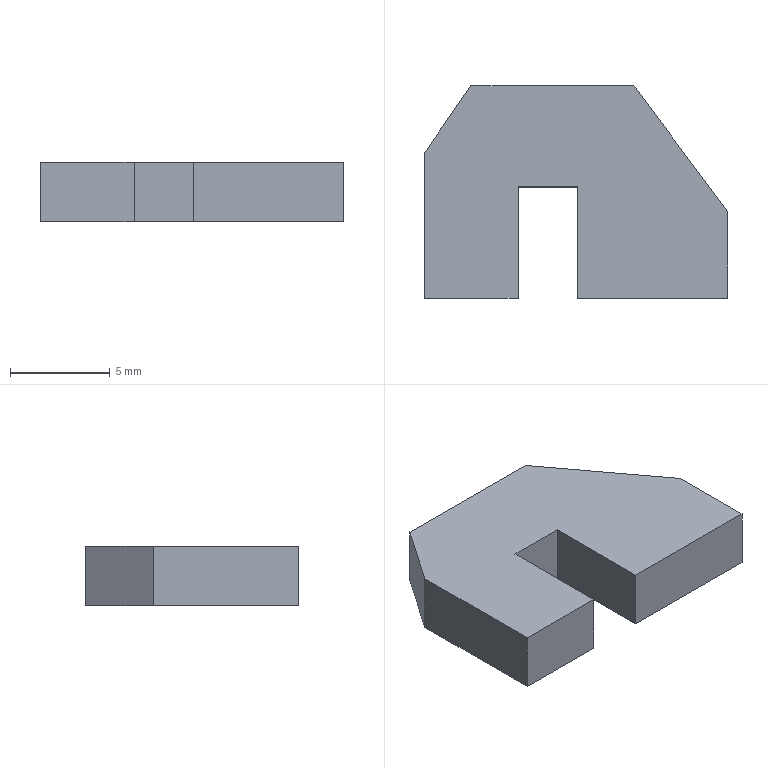Part | SolidWorks | features BaseBody 1 | 1 solid | 12 faces | box 15.248 x 10.684 x 3 mm | volume 381.769 mm3 | plane 10 | spline 2
STEP:
#1=CARTESIAN_POINT('',(96.385,5.305,-1.5));
#2=VERTEX_POINT('',#1);
#3=CARTESIAN_POINT('',(96.385,10.901,-1.5));
#4=VERTEX_POINT('',#3);
#5=CARTESIAN_POINT('',(96.385,0.,-1.5));
#6=DIRECTION('',(0.,1.,0.));
#7=VECTOR('',#6,1000.);
#8=LINE('',#5,#7);
#9=EDGE_CURVE('',#2,#4,#8,.T.);
#10=ORIENTED_EDGE('',*,*,#9,.T.);
#11=CARTESIAN_POINT('',(93.391,10.901,-1.5));
#12=VERTEX_POINT('',#11);
#13=CARTESIAN_POINT('',(0.,10.901,-1.5));
#14=DIRECTION('',(-1.,0.,0.));
#15=VECTOR('',#14,1000.);
#16=LINE('',#13,#15);
#17=EDGE_CURVE('',#4,#12,#16,.T.);
#18=ORIENTED_EDGE('',*,*,#17,.T.);
#19=CARTESIAN_POINT('',(93.391,5.305,-1.5));
#20=VERTEX_POINT('',#19);
#21=CARTESIAN_POINT('',(93.391,0.,-1.5));
#22=DIRECTION('',(0.,-1.,0.));
#23=VECTOR('',#22,1000.);
#24=LINE('',#21,#23);
#25=EDGE_CURVE('',#12,#20,#24,.T.);
#26=ORIENTED_EDGE('',*,*,#25,.T.);
#27=CARTESIAN_POINT('',(88.677,5.305,-1.5));
#28=VERTEX_POINT('',#27);
#29=CARTESIAN_POINT('',(0.,5.305,-1.5));
#30=DIRECTION('',(1.,0.,0.));
#31=VECTOR('',#30,1000.);
#32=LINE('',#29,#31);
#33=EDGE_CURVE('',#28,#20,#32,.T.);
#34=ORIENTED_EDGE('',*,*,#33,.F.);
#35=CARTESIAN_POINT('',(88.677,12.595,-1.5));
#36=VERTEX_POINT('',#35);
#37=CARTESIAN_POINT('',(88.677,0.,-1.5));
#38=DIRECTION('',(0.,-1.,0.));
#39=VECTOR('',#38,1000.);
#40=LINE('',#37,#39);
#41=EDGE_CURVE('',#36,#28,#40,.T.);
#42=ORIENTED_EDGE('',*,*,#41,.F.);
#43=CARTESIAN_POINT('',(91.019,15.989,-1.5));
#44=VERTEX_POINT('',#43);
#45=CARTESIAN_POINT('',(91.019,15.989,-1.5));
#46=CARTESIAN_POINT('',(90.238,14.856,-1.5));
#47=CARTESIAN_POINT('',(89.458,13.725,-1.5));
#48=CARTESIAN_POINT('',(88.677,12.595,-1.5));
#49=B_SPLINE_CURVE_WITH_KNOTS('',3,(#45,#46,#47,#48),.UNSPECIFIED.,.F.,.F.,(4,4),(0.7273,0.8182),.UNSPECIFIED.);
#50=EDGE_CURVE('',#44,#36,#49,.T.);
#51=ORIENTED_EDGE('',*,*,#50,.F.);
#52=CARTESIAN_POINT('',(99.205,15.989,-1.5));
#53=VERTEX_POINT('',#52);
#54=CARTESIAN_POINT('',(0.,15.989,-1.5));
#55=DIRECTION('',(-1.,0.,0.));
#56=VECTOR('',#55,1000.);
#57=LINE('',#54,#56);
#58=EDGE_CURVE('',#53,#44,#57,.T.);
#59=ORIENTED_EDGE('',*,*,#58,.F.);
#60=CARTESIAN_POINT('',(103.925,9.662,-1.5));
#61=VERTEX_POINT('',#60);
#62=CARTESIAN_POINT('',(103.925,9.662,-1.5));
#63=CARTESIAN_POINT('',(102.352,11.771,-1.5));
#64=CARTESIAN_POINT('',(100.779,13.879,-1.5));
#65=CARTESIAN_POINT('',(99.205,15.989,-1.5));
#66=B_SPLINE_CURVE_WITH_KNOTS('',3,(#62,#63,#64,#65),.UNSPECIFIED.,.F.,.F.,(4,4),(0.5455,0.6364),.UNSPECIFIED.);
#67=EDGE_CURVE('',#61,#53,#66,.T.);
#68=ORIENTED_EDGE('',*,*,#67,.F.);
#69=CARTESIAN_POINT('',(103.925,5.305,-1.5));
#70=VERTEX_POINT('',#69);
#71=CARTESIAN_POINT('',(103.925,0.,-1.5));
#72=DIRECTION('',(0.,1.,0.));
#73=VECTOR('',#72,1000.);
#74=LINE('',#71,#73);
#75=EDGE_CURVE('',#70,#61,#74,.T.);
#76=ORIENTED_EDGE('',*,*,#75,.F.);
#77=CARTESIAN_POINT('',(0.,5.305,-1.5));
#78=DIRECTION('',(1.,0.,0.));
#79=VECTOR('',#78,1000.);
#80=LINE('',#77,#79);
#81=EDGE_CURVE('',#2,#70,#80,.T.);
#82=ORIENTED_EDGE('',*,*,#81,.F.);
#83=EDGE_LOOP('',(#10,#18,#26,#34,#42,#51,#59,#68,#76,#82));
#84=FACE_OUTER_BOUND('',#83,.T.);
#85=CARTESIAN_POINT('',(0.,0.,-1.5));
#86=DIRECTION('',(0.,0.,1.));
#87=DIRECTION('',(1.,0.,0.));
#88=AXIS2_PLACEMENT_3D('',#85,#86,#87);
#89=PLANE('',#88);
#90=ADVANCED_FACE('',(#84),#89,.F.);
#91=CARTESIAN_POINT('',(96.385,5.305,1.5));
#92=VERTEX_POINT('',#91);
#93=CARTESIAN_POINT('',(96.385,10.901,1.5));
#94=VERTEX_POINT('',#93);
#95=CARTESIAN_POINT('',(96.385,0.,1.5));
#96=DIRECTION('',(0.,1.,0.));
#97=VECTOR('',#96,1000.);
#98=LINE('',#95,#97);
#99=EDGE_CURVE('',#92,#94,#98,.T.);
#100=ORIENTED_EDGE('',*,*,#99,.F.);
#101=CARTESIAN_POINT('',(103.925,5.305,1.5));
#102=VERTEX_POINT('',#101);
#103=CARTESIAN_POINT('',(0.,5.305,1.5));
#104=DIRECTION('',(1.,0.,0.));
#105=VECTOR('',#104,1000.);
#106=LINE('',#103,#105);
#107=EDGE_CURVE('',#92,#102,#106,.T.);
#108=ORIENTED_EDGE('',*,*,#107,.T.);
#109=CARTESIAN_POINT('',(103.925,9.662,1.5));
#110=VERTEX_POINT('',#109);
#111=CARTESIAN_POINT('',(103.925,0.,1.5));
#112=DIRECTION('',(0.,1.,0.));
#113=VECTOR('',#112,1000.);
#114=LINE('',#111,#113);
#115=EDGE_CURVE('',#102,#110,#114,.T.);
#116=ORIENTED_EDGE('',*,*,#115,.T.);
#117=CARTESIAN_POINT('',(99.205,15.989,1.5));
#118=VERTEX_POINT('',#117);
#119=CARTESIAN_POINT('',(103.925,9.662,1.5));
#120=CARTESIAN_POINT('',(102.352,11.771,1.5));
#121=CARTESIAN_POINT('',(100.779,13.879,1.5));
#122=CARTESIAN_POINT('',(99.205,15.989,1.5));
#123=B_SPLINE_CURVE_WITH_KNOTS('',3,(#119,#120,#121,#122),.UNSPECIFIED.,.F.,.F.,(4,4),(0.5455,0.6364),.UNSPECIFIED.);
#124=EDGE_CURVE('',#110,#118,#123,.T.);
#125=ORIENTED_EDGE('',*,*,#124,.T.);
#126=CARTESIAN_POINT('',(91.019,15.989,1.5));
#127=VERTEX_POINT('',#126);
#128=CARTESIAN_POINT('',(0.,15.989,1.5));
#129=DIRECTION('',(-1.,0.,0.));
#130=VECTOR('',#129,1000.);
#131=LINE('',#128,#130);
#132=EDGE_CURVE('',#118,#127,#131,.T.);
#133=ORIENTED_EDGE('',*,*,#132,.T.);
#134=CARTESIAN_POINT('',(88.677,12.595,1.5));
#135=VERTEX_POINT('',#134);
#136=CARTESIAN_POINT('',(91.019,15.989,1.5));
#137=CARTESIAN_POINT('',(90.238,14.856,1.5));
#138=CARTESIAN_POINT('',(89.458,13.725,1.5));
#139=CARTESIAN_POINT('',(88.677,12.595,1.5));
#140=B_SPLINE_CURVE_WITH_KNOTS('',3,(#136,#137,#138,#139),.UNSPECIFIED.,.F.,.F.,(4,4),(0.7273,0.8182),.UNSPECIFIED.);
#141=EDGE_CURVE('',#127,#135,#140,.T.);
#142=ORIENTED_EDGE('',*,*,#141,.T.);
#143=CARTESIAN_POINT('',(88.677,5.305,1.5));
#144=VERTEX_POINT('',#143);
#145=CARTESIAN_POINT('',(88.677,0.,1.5));
#146=DIRECTION('',(0.,-1.,0.));
#147=VECTOR('',#146,1000.);
#148=LINE('',#145,#147);
#149=EDGE_CURVE('',#135,#144,#148,.T.);
#150=ORIENTED_EDGE('',*,*,#149,.T.);
#151=CARTESIAN_POINT('',(93.391,5.305,1.5));
#152=VERTEX_POINT('',#151);
#153=CARTESIAN_POINT('',(0.,5.305,1.5));
#154=DIRECTION('',(1.,0.,0.));
#155=VECTOR('',#154,1000.);
#156=LINE('',#153,#155);
#157=EDGE_CURVE('',#144,#152,#156,.T.);
#158=ORIENTED_EDGE('',*,*,#157,.T.);
#159=CARTESIAN_POINT('',(93.391,10.901,1.5));
#160=VERTEX_POINT('',#159);
#161=CARTESIAN_POINT('',(93.391,0.,1.5));
#162=DIRECTION('',(0.,-1.,0.));
#163=VECTOR('',#162,1000.);
#164=LINE('',#161,#163);
#165=EDGE_CURVE('',#160,#152,#164,.T.);
#166=ORIENTED_EDGE('',*,*,#165,.F.);
#167=CARTESIAN_POINT('',(0.,10.901,1.5));
#168=DIRECTION('',(-1.,0.,0.));
#169=VECTOR('',#168,1000.);
#170=LINE('',#167,#169);
#171=EDGE_CURVE('',#94,#160,#170,.T.);
#172=ORIENTED_EDGE('',*,*,#171,.F.);
#173=EDGE_LOOP('',(#100,#108,#116,#125,#133,#142,#150,#158,#166,#172));
#174=FACE_OUTER_BOUND('',#173,.T.);
#175=CARTESIAN_POINT('',(0.,0.,1.5));
#176=DIRECTION('',(0.,0.,1.));
#177=DIRECTION('',(1.,0.,0.));
#178=AXIS2_PLACEMENT_3D('',#175,#176,#177);
#179=PLANE('',#178);
#180=ADVANCED_FACE('',(#174),#179,.T.);
#181=ORIENTED_EDGE('',*,*,#17,.F.);
#182=CARTESIAN_POINT('',(96.385,10.901,1.5));
#183=DIRECTION('',(0.,0.,-1.));
#184=VECTOR('',#183,1000.);
#185=LINE('',#182,#184);
#186=EDGE_CURVE('',#94,#4,#185,.T.);
#187=ORIENTED_EDGE('',*,*,#186,.F.);
#188=ORIENTED_EDGE('',*,*,#171,.T.);
#189=CARTESIAN_POINT('',(93.391,10.901,1.5));
#190=DIRECTION('',(0.,0.,-1.));
#191=VECTOR('',#190,1000.);
#192=LINE('',#189,#191);
#193=EDGE_CURVE('',#160,#12,#192,.T.);
#194=ORIENTED_EDGE('',*,*,#193,.T.);
#195=EDGE_LOOP('',(#181,#187,#188,#194));
#196=FACE_OUTER_BOUND('',#195,.T.);
#197=CARTESIAN_POINT('',(0.,10.901,1.5));
#198=DIRECTION('',(0.,-1.,0.));
#199=DIRECTION('',(0.,0.,-1.));
#200=AXIS2_PLACEMENT_3D('',#197,#198,#199);
#201=PLANE('',#200);
#202=ADVANCED_FACE('',(#196),#201,.T.);
#203=ORIENTED_EDGE('',*,*,#25,.F.);
#204=ORIENTED_EDGE('',*,*,#193,.F.);
#205=ORIENTED_EDGE('',*,*,#165,.T.);
#206=CARTESIAN_POINT('',(93.391,5.305,1.5));
#207=DIRECTION('',(0.,0.,-1.));
#208=VECTOR('',#207,1000.);
#209=LINE('',#206,#208);
#210=EDGE_CURVE('',#152,#20,#209,.T.);
#211=ORIENTED_EDGE('',*,*,#210,.T.);
#212=EDGE_LOOP('',(#203,#204,#205,#211));
#213=FACE_OUTER_BOUND('',#212,.T.);
#214=CARTESIAN_POINT('',(93.391,0.,1.5));
#215=DIRECTION('',(1.,0.,0.));
#216=DIRECTION('',(0.,1.,0.));
#217=AXIS2_PLACEMENT_3D('',#214,#215,#216);
#218=PLANE('',#217);
#219=ADVANCED_FACE('',(#213),#218,.T.);
#220=ORIENTED_EDGE('',*,*,#33,.T.);
#221=ORIENTED_EDGE('',*,*,#210,.F.);
#222=ORIENTED_EDGE('',*,*,#157,.F.);
#223=CARTESIAN_POINT('',(88.677,5.305,1.5));
#224=DIRECTION('',(0.,0.,-1.));
#225=VECTOR('',#224,1000.);
#226=LINE('',#223,#225);
#227=EDGE_CURVE('',#144,#28,#226,.T.);
#228=ORIENTED_EDGE('',*,*,#227,.T.);
#229=EDGE_LOOP('',(#220,#221,#222,#228));
#230=FACE_OUTER_BOUND('',#229,.T.);
#231=CARTESIAN_POINT('',(0.,5.305,1.5));
#232=DIRECTION('',(0.,1.,0.));
#233=DIRECTION('',(1.,0.,0.));
#234=AXIS2_PLACEMENT_3D('',#231,#232,#233);
#235=PLANE('',#234);
#236=ADVANCED_FACE('',(#230),#235,.F.);
#237=ORIENTED_EDGE('',*,*,#41,.T.);
#238=ORIENTED_EDGE('',*,*,#227,.F.);
#239=ORIENTED_EDGE('',*,*,#149,.F.);
#240=CARTESIAN_POINT('',(88.677,12.595,1.5));
#241=DIRECTION('',(0.,0.,-1.));
#242=VECTOR('',#241,1000.);
#243=LINE('',#240,#242);
#244=EDGE_CURVE('',#135,#36,#243,.T.);
#245=ORIENTED_EDGE('',*,*,#244,.T.);
#246=EDGE_LOOP('',(#237,#238,#239,#245));
#247=FACE_OUTER_BOUND('',#246,.T.);
#248=CARTESIAN_POINT('',(88.677,0.,1.5));
#249=DIRECTION('',(1.,0.,0.));
#250=DIRECTION('',(0.,1.,0.));
#251=AXIS2_PLACEMENT_3D('',#248,#249,#250);
#252=PLANE('',#251);
#253=ADVANCED_FACE('',(#247),#252,.F.);
#254=ORIENTED_EDGE('',*,*,#50,.T.);
#255=ORIENTED_EDGE('',*,*,#244,.F.);
#256=ORIENTED_EDGE('',*,*,#141,.F.);
#257=CARTESIAN_POINT('',(91.019,15.989,1.5));
#258=DIRECTION('',(0.,0.,-1.));
#259=VECTOR('',#258,1000.);
#260=LINE('',#257,#259);
#261=EDGE_CURVE('',#127,#44,#260,.T.);
#262=ORIENTED_EDGE('',*,*,#261,.T.);
#263=EDGE_LOOP('',(#254,#255,#256,#262));
#264=FACE_OUTER_BOUND('',#263,.T.);
#265=CARTESIAN_POINT('',(91.019,15.989,1.5));
#266=CARTESIAN_POINT('',(91.019,15.989,-1.5));
#267=CARTESIAN_POINT('',(90.238,14.856,1.5));
#268=CARTESIAN_POINT('',(90.238,14.856,-1.5));
#269=CARTESIAN_POINT('',(89.458,13.725,1.5));
#270=CARTESIAN_POINT('',(89.458,13.725,-1.5));
#271=CARTESIAN_POINT('',(88.677,12.595,1.5));
#272=CARTESIAN_POINT('',(88.677,12.595,-1.5));
#273=B_SPLINE_SURFACE_WITH_KNOTS('',3,1,((#265,#266),(#267,#268),(#269,#270),(#271,#272)),.UNSPECIFIED.,.F.,.F.,.F.,(4,4),(2,2),(0.7273,0.8182),(0.,1.),.UNSPECIFIED.);
#274=ADVANCED_FACE('',(#264),#273,.F.);
#275=ORIENTED_EDGE('',*,*,#58,.T.);
#276=ORIENTED_EDGE('',*,*,#261,.F.);
#277=ORIENTED_EDGE('',*,*,#132,.F.);
#278=CARTESIAN_POINT('',(99.205,15.989,1.5));
#279=DIRECTION('',(0.,0.,-1.));
#280=VECTOR('',#279,1000.);
#281=LINE('',#278,#280);
#282=EDGE_CURVE('',#118,#53,#281,.T.);
#283=ORIENTED_EDGE('',*,*,#282,.T.);
#284=EDGE_LOOP('',(#275,#276,#277,#283));
#285=FACE_OUTER_BOUND('',#284,.T.);
#286=CARTESIAN_POINT('',(0.,15.989,1.5));
#287=DIRECTION('',(0.,-1.,0.));
#288=DIRECTION('',(0.,0.,-1.));
#289=AXIS2_PLACEMENT_3D('',#286,#287,#288);
#290=PLANE('',#289);
#291=ADVANCED_FACE('',(#285),#290,.F.);
#292=ORIENTED_EDGE('',*,*,#67,.T.);
#293=ORIENTED_EDGE('',*,*,#282,.F.);
#294=ORIENTED_EDGE('',*,*,#124,.F.);
#295=CARTESIAN_POINT('',(103.925,9.662,1.5));
#296=DIRECTION('',(0.,0.,-1.));
#297=VECTOR('',#296,1000.);
#298=LINE('',#295,#297);
#299=EDGE_CURVE('',#110,#61,#298,.T.);
#300=ORIENTED_EDGE('',*,*,#299,.T.);
#301=EDGE_LOOP('',(#292,#293,#294,#300));
#302=FACE_OUTER_BOUND('',#301,.T.);
#303=CARTESIAN_POINT('',(103.925,9.662,1.5));
#304=CARTESIAN_POINT('',(103.925,9.662,-1.5));
#305=CARTESIAN_POINT('',(102.352,11.771,1.5));
#306=CARTESIAN_POINT('',(102.352,11.771,-1.5));
#307=CARTESIAN_POINT('',(100.779,13.879,1.5));
#308=CARTESIAN_POINT('',(100.779,13.879,-1.5));
#309=CARTESIAN_POINT('',(99.205,15.989,1.5));
#310=CARTESIAN_POINT('',(99.205,15.989,-1.5));
#311=B_SPLINE_SURFACE_WITH_KNOTS('',3,1,((#303,#304),(#305,#306),(#307,#308),(#309,#310)),.UNSPECIFIED.,.F.,.F.,.F.,(4,4),(2,2),(0.5455,0.6364),(0.,1.),.UNSPECIFIED.);
#312=ADVANCED_FACE('',(#302),#311,.F.);
#313=ORIENTED_EDGE('',*,*,#75,.T.);
#314=ORIENTED_EDGE('',*,*,#299,.F.);
#315=ORIENTED_EDGE('',*,*,#115,.F.);
#316=CARTESIAN_POINT('',(103.925,5.305,1.5));
#317=DIRECTION('',(0.,0.,-1.));
#318=VECTOR('',#317,1000.);
#319=LINE('',#316,#318);
#320=EDGE_CURVE('',#102,#70,#319,.T.);
#321=ORIENTED_EDGE('',*,*,#320,.T.);
#322=EDGE_LOOP('',(#313,#314,#315,#321));
#323=FACE_OUTER_BOUND('',#322,.T.);
#324=CARTESIAN_POINT('',(103.925,0.,1.5));
#325=DIRECTION('',(-1.,0.,0.));
#326=DIRECTION('',(0.,0.,1.));
#327=AXIS2_PLACEMENT_3D('',#324,#325,#326);
#328=PLANE('',#327);
#329=ADVANCED_FACE('',(#323),#328,.F.);
#330=ORIENTED_EDGE('',*,*,#81,.T.);
#331=ORIENTED_EDGE('',*,*,#320,.F.);
#332=ORIENTED_EDGE('',*,*,#107,.F.);
#333=CARTESIAN_POINT('',(96.385,5.305,1.5));
#334=DIRECTION('',(0.,0.,-1.));
#335=VECTOR('',#334,1000.);
#336=LINE('',#333,#335);
#337=EDGE_CURVE('',#92,#2,#336,.T.);
#338=ORIENTED_EDGE('',*,*,#337,.T.);
#339=EDGE_LOOP('',(#330,#331,#332,#338));
#340=FACE_OUTER_BOUND('',#339,.T.);
#341=CARTESIAN_POINT('',(0.,5.305,1.5));
#342=DIRECTION('',(0.,1.,0.));
#343=DIRECTION('',(1.,0.,0.));
#344=AXIS2_PLACEMENT_3D('',#341,#342,#343);
#345=PLANE('',#344);
#346=ADVANCED_FACE('',(#340),#345,.F.);
#347=ORIENTED_EDGE('',*,*,#9,.F.);
#348=ORIENTED_EDGE('',*,*,#337,.F.);
#349=ORIENTED_EDGE('',*,*,#99,.T.);
#350=ORIENTED_EDGE('',*,*,#186,.T.);
#351=EDGE_LOOP('',(#347,#348,#349,#350));
#352=FACE_OUTER_BOUND('',#351,.T.);
#353=CARTESIAN_POINT('',(96.385,0.,1.5));
#354=DIRECTION('',(-1.,0.,0.));
#355=DIRECTION('',(0.,1.,0.));
#356=AXIS2_PLACEMENT_3D('',#353,#354,#355);
#357=PLANE('',#356);
#358=ADVANCED_FACE('',(#352),#357,.T.);
#359=CLOSED_SHELL('',(#90,#180,#202,#219,#236,#253,#274,#291,#312,#329,#346,#358));
#360=MANIFOLD_SOLID_BREP('',#359);
#361=CARTESIAN_POINT('',(0.,0.,0.));
#362=DIRECTION('',(0.,0.,1.));
#363=DIRECTION('',(1.,0.,0.));
#364=AXIS2_PLACEMENT_3D('',#361,#362,#363);
#365=(LENGTH_UNIT()NAMED_UNIT(*)SI_UNIT(.MILLI.,.METRE.));
#366=UNCERTAINTY_MEASURE_WITH_UNIT(LENGTH_MEASURE(0.00001),#365,'','');
#367=(NAMED_UNIT(*)PLANE_ANGLE_UNIT()SI_UNIT($,.RADIAN.));
#368=(NAMED_UNIT(*)SI_UNIT($,.STERADIAN.)SOLID_ANGLE_UNIT());
#369=(GEOMETRIC_REPRESENTATION_CONTEXT(3)GLOBAL_UNCERTAINTY_ASSIGNED_CONTEXT((#366))GLOBAL_UNIT_ASSIGNED_CONTEXT((#365,#367,#368))REPRESENTATION_CONTEXT('',''));
#370=ADVANCED_BREP_SHAPE_REPRESENTATION('',(#360,#364),#369);